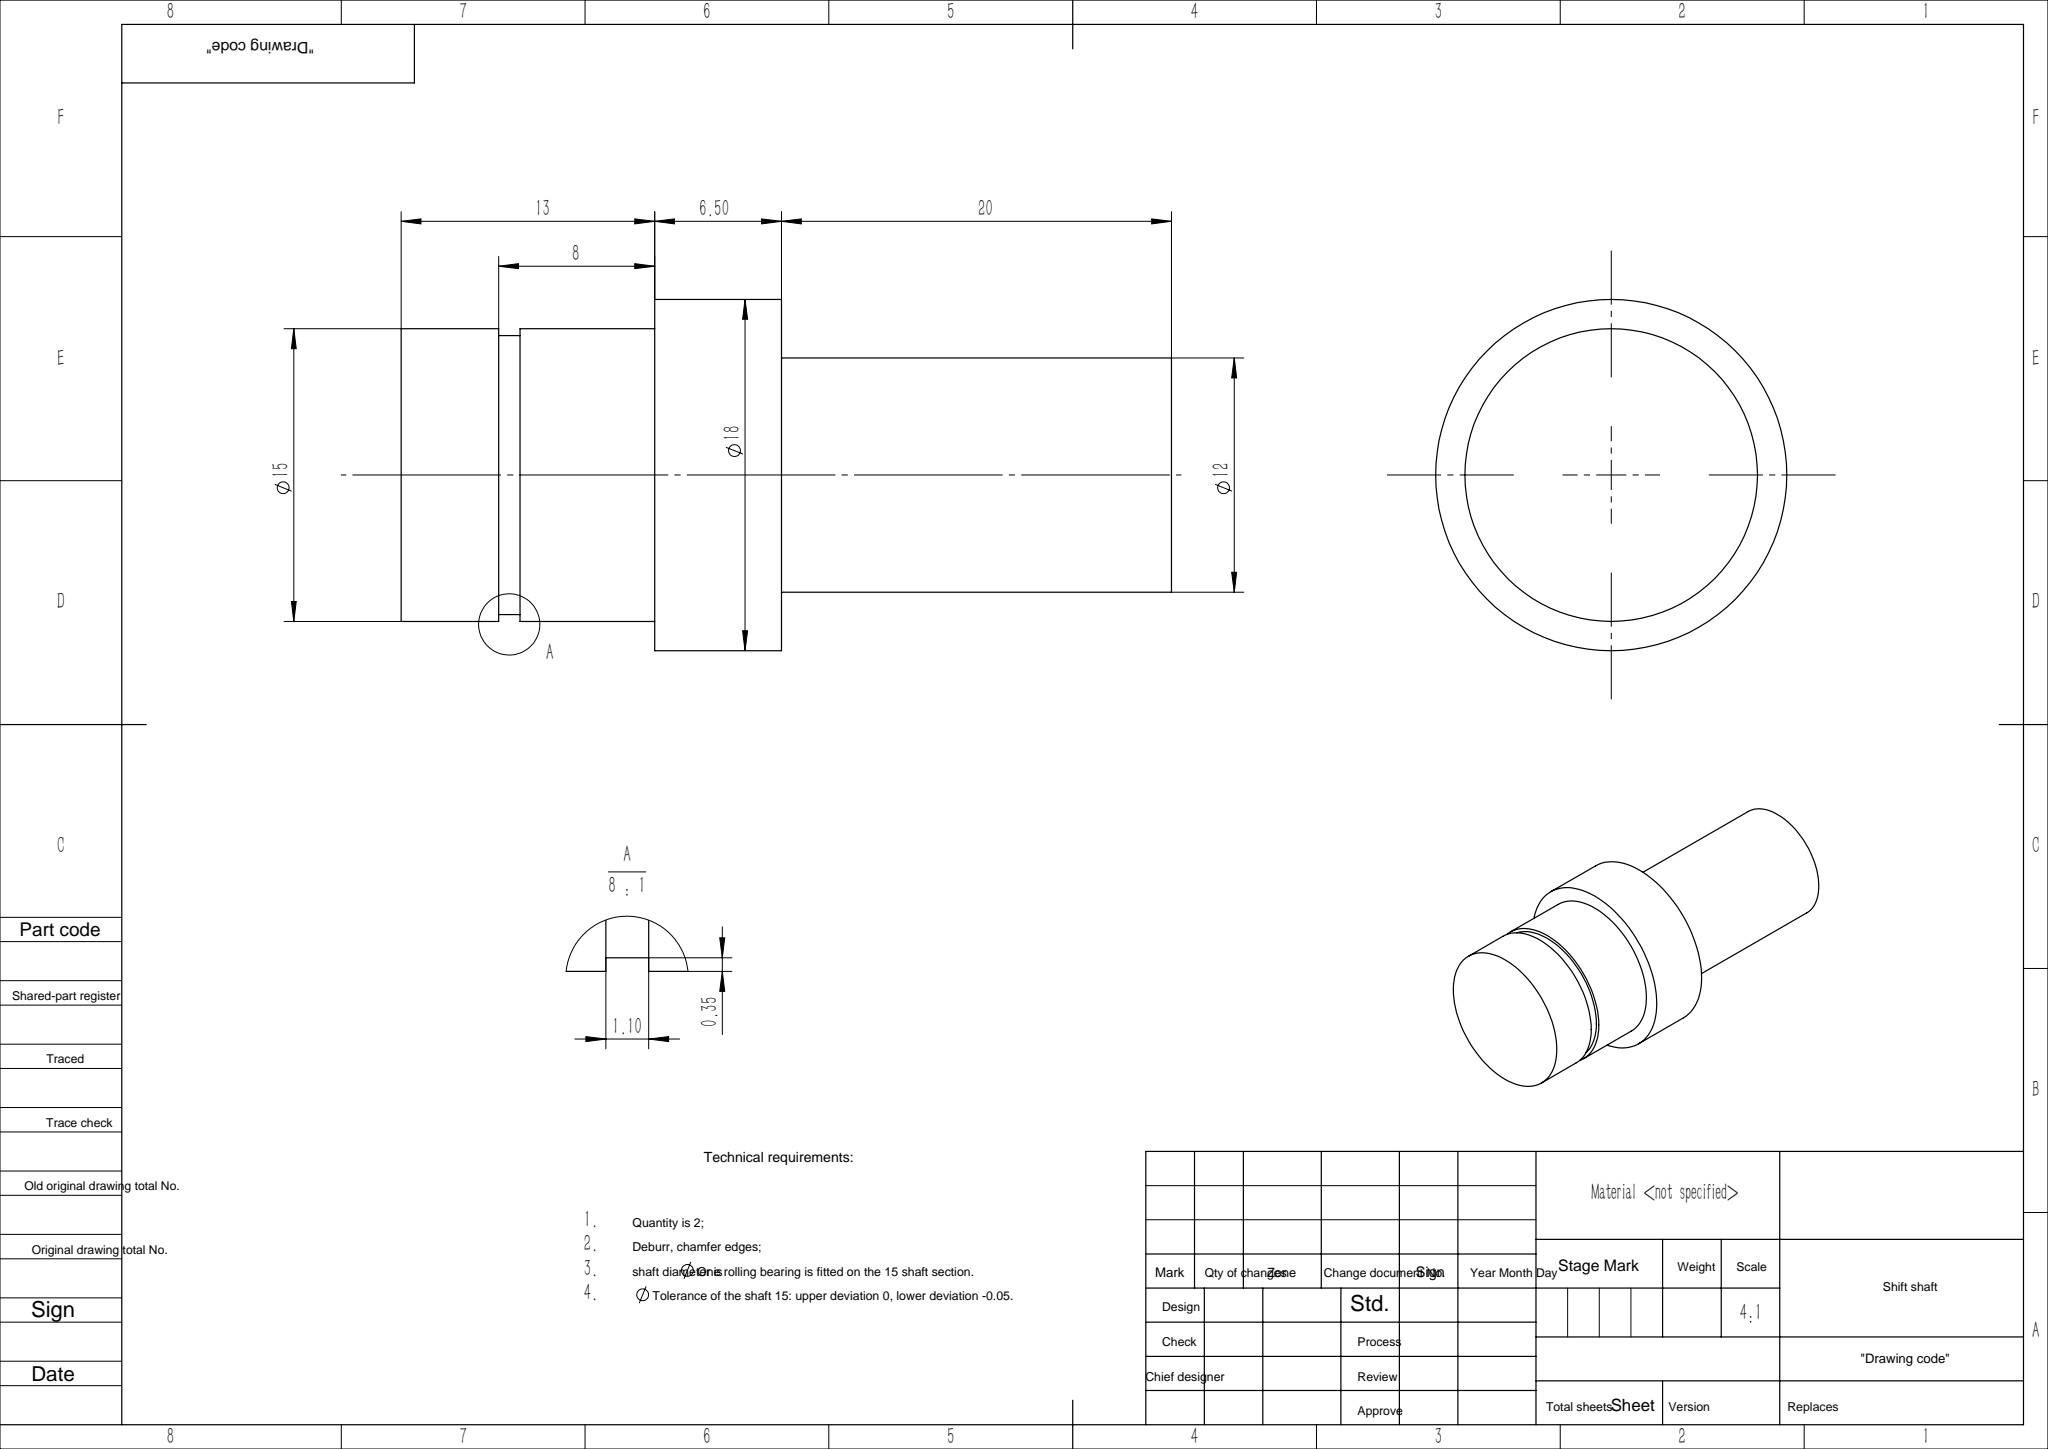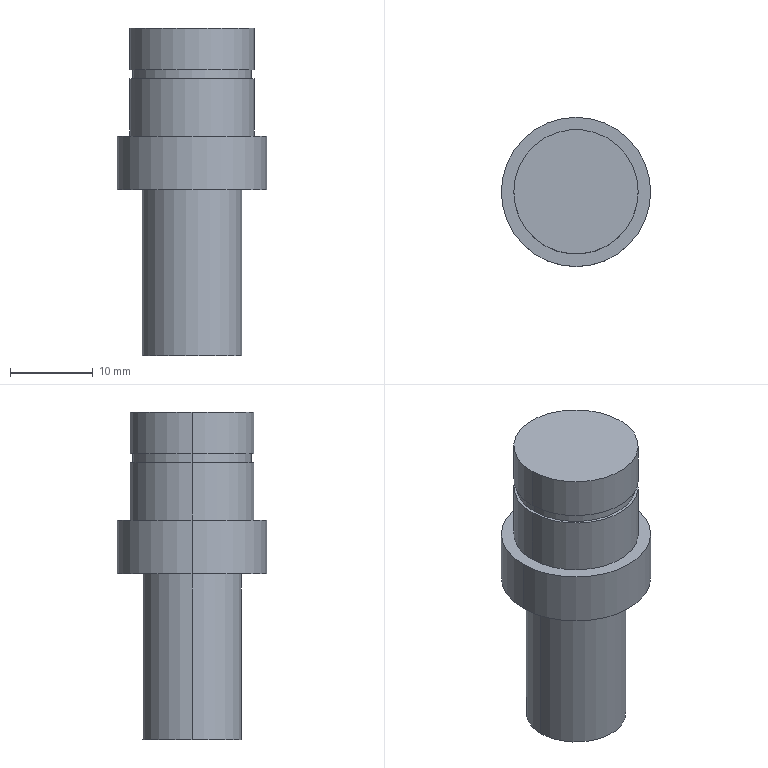Part | SolidWorks | features ICE 1, Revolution 1 | 1 solid | 16 faces | box 18 x 18 x 39.5 mm | volume 6196 mm3 | cylinder 10 | plane 6 | commonest cylinder face diameters 15 x4 12 x2 14.3 x2 18 x2
STEP:
#1=CARTESIAN_POINT('',(-7.5,0.,0.));
#2=VERTEX_POINT('',#1);
#3=CARTESIAN_POINT('',(7.5,0.,0.));
#4=VERTEX_POINT('',#3);
#5=CARTESIAN_POINT('',(0.,0.,0.));
#6=DIRECTION('',(0.,0.,-1.));
#7=DIRECTION('',(-1.,0.,0.));
#8=AXIS2_PLACEMENT_3D('',#5,#6,#7);
#9=CIRCLE('',#8,7.5);
#10=EDGE_CURVE('',#2,#4,#9,.T.);
#11=ORIENTED_EDGE('',*,*,#10,.T.);
#12=CARTESIAN_POINT('',(7.5,0.,-5.));
#13=VERTEX_POINT('',#12);
#14=CARTESIAN_POINT('',(7.5,0.,-39.5));
#15=DIRECTION('',(0.,0.,-1.));
#16=VECTOR('',#15,1000.);
#17=LINE('',#14,#16);
#18=EDGE_CURVE('',#4,#13,#17,.T.);
#19=ORIENTED_EDGE('',*,*,#18,.T.);
#20=CARTESIAN_POINT('',(-7.5,0.,-5.));
#21=VERTEX_POINT('',#20);
#22=CARTESIAN_POINT('',(0.,0.,-5.));
#23=DIRECTION('',(0.,0.,1.));
#24=DIRECTION('',(1.,0.,0.));
#25=AXIS2_PLACEMENT_3D('',#22,#23,#24);
#26=CIRCLE('',#25,7.5);
#27=EDGE_CURVE('',#13,#21,#26,.T.);
#28=ORIENTED_EDGE('',*,*,#27,.T.);
#29=CARTESIAN_POINT('',(-7.5,0.,-39.5));
#30=DIRECTION('',(0.,0.,-1.));
#31=VECTOR('',#30,1000.);
#32=LINE('',#29,#31);
#33=EDGE_CURVE('',#2,#21,#32,.T.);
#34=ORIENTED_EDGE('',*,*,#33,.F.);
#35=EDGE_LOOP('',(#11,#19,#28,#34));
#36=FACE_OUTER_BOUND('',#35,.T.);
#37=CARTESIAN_POINT('',(0.,0.,-39.5));
#38=DIRECTION('',(0.,0.,-1.));
#39=DIRECTION('',(-1.,0.,0.));
#40=AXIS2_PLACEMENT_3D('',#37,#38,#39);
#41=CYLINDRICAL_SURFACE('',#40,7.5);
#42=ADVANCED_FACE('',(#36),#41,.T.);
#43=CARTESIAN_POINT('',(7.15,0.,-6.1));
#44=VERTEX_POINT('',#43);
#45=CARTESIAN_POINT('',(-7.15,0.,-6.1));
#46=VERTEX_POINT('',#45);
#47=CARTESIAN_POINT('',(0.,0.,-6.1));
#48=DIRECTION('',(0.,0.,1.));
#49=DIRECTION('',(1.,0.,0.));
#50=AXIS2_PLACEMENT_3D('',#47,#48,#49);
#51=CIRCLE('',#50,7.15);
#52=EDGE_CURVE('',#44,#46,#51,.T.);
#53=ORIENTED_EDGE('',*,*,#52,.T.);
#54=CARTESIAN_POINT('',(-7.15,0.,-5.));
#55=VERTEX_POINT('',#54);
#56=CARTESIAN_POINT('',(-7.15,0.,-6.1));
#57=DIRECTION('',(0.,0.,1.));
#58=VECTOR('',#57,1000.);
#59=LINE('',#56,#58);
#60=EDGE_CURVE('',#46,#55,#59,.T.);
#61=ORIENTED_EDGE('',*,*,#60,.T.);
#62=CARTESIAN_POINT('',(7.15,0.,-5.));
#63=VERTEX_POINT('',#62);
#64=CARTESIAN_POINT('',(0.,0.,-5.));
#65=DIRECTION('',(0.,0.,1.));
#66=DIRECTION('',(1.,0.,0.));
#67=AXIS2_PLACEMENT_3D('',#64,#65,#66);
#68=CIRCLE('',#67,7.15);
#69=EDGE_CURVE('',#63,#55,#68,.T.);
#70=ORIENTED_EDGE('',*,*,#69,.F.);
#71=CARTESIAN_POINT('',(7.15,0.,-6.1));
#72=DIRECTION('',(0.,0.,1.));
#73=VECTOR('',#72,1000.);
#74=LINE('',#71,#73);
#75=EDGE_CURVE('',#44,#63,#74,.T.);
#76=ORIENTED_EDGE('',*,*,#75,.F.);
#77=EDGE_LOOP('',(#53,#61,#70,#76));
#78=FACE_OUTER_BOUND('',#77,.T.);
#79=CARTESIAN_POINT('',(0.,0.,-6.1));
#80=DIRECTION('',(0.,0.,1.));
#81=DIRECTION('',(1.,0.,0.));
#82=AXIS2_PLACEMENT_3D('',#79,#80,#81);
#83=CYLINDRICAL_SURFACE('',#82,7.15);
#84=ADVANCED_FACE('',(#78),#83,.T.);
#85=CARTESIAN_POINT('',(-6.,0.,-19.5));
#86=VERTEX_POINT('',#85);
#87=CARTESIAN_POINT('',(6.,0.,-19.5));
#88=VERTEX_POINT('',#87);
#89=CARTESIAN_POINT('',(0.,0.,-19.5));
#90=DIRECTION('',(0.,0.,-1.));
#91=DIRECTION('',(-1.,0.,0.));
#92=AXIS2_PLACEMENT_3D('',#89,#90,#91);
#93=CIRCLE('',#92,6.);
#94=EDGE_CURVE('',#86,#88,#93,.T.);
#95=ORIENTED_EDGE('',*,*,#94,.T.);
#96=CARTESIAN_POINT('',(6.,0.,-39.5));
#97=VERTEX_POINT('',#96);
#98=CARTESIAN_POINT('',(6.,0.,-39.5));
#99=DIRECTION('',(0.,0.,-1.));
#100=VECTOR('',#99,1000.);
#101=LINE('',#98,#100);
#102=EDGE_CURVE('',#88,#97,#101,.T.);
#103=ORIENTED_EDGE('',*,*,#102,.T.);
#104=CARTESIAN_POINT('',(-6.,0.,-39.5));
#105=VERTEX_POINT('',#104);
#106=CARTESIAN_POINT('',(0.,0.,-39.5));
#107=DIRECTION('',(0.,0.,-1.));
#108=DIRECTION('',(-1.,0.,0.));
#109=AXIS2_PLACEMENT_3D('',#106,#107,#108);
#110=CIRCLE('',#109,6.);
#111=EDGE_CURVE('',#105,#97,#110,.T.);
#112=ORIENTED_EDGE('',*,*,#111,.F.);
#113=CARTESIAN_POINT('',(-6.,0.,-39.5));
#114=DIRECTION('',(0.,0.,-1.));
#115=VECTOR('',#114,1000.);
#116=LINE('',#113,#115);
#117=EDGE_CURVE('',#86,#105,#116,.T.);
#118=ORIENTED_EDGE('',*,*,#117,.F.);
#119=EDGE_LOOP('',(#95,#103,#112,#118));
#120=FACE_OUTER_BOUND('',#119,.T.);
#121=CARTESIAN_POINT('',(0.,0.,-39.5));
#122=DIRECTION('',(0.,0.,-1.));
#123=DIRECTION('',(-1.,0.,0.));
#124=AXIS2_PLACEMENT_3D('',#121,#122,#123);
#125=CYLINDRICAL_SURFACE('',#124,6.);
#126=ADVANCED_FACE('',(#120),#125,.T.);
#127=CARTESIAN_POINT('',(-9.,0.,-13.));
#128=VERTEX_POINT('',#127);
#129=CARTESIAN_POINT('',(9.,0.,-13.));
#130=VERTEX_POINT('',#129);
#131=CARTESIAN_POINT('',(0.,0.,-13.));
#132=DIRECTION('',(0.,0.,-1.));
#133=DIRECTION('',(-1.,0.,0.));
#134=AXIS2_PLACEMENT_3D('',#131,#132,#133);
#135=CIRCLE('',#134,9.);
#136=EDGE_CURVE('',#128,#130,#135,.T.);
#137=ORIENTED_EDGE('',*,*,#136,.T.);
#138=CARTESIAN_POINT('',(9.,0.,-19.5));
#139=VERTEX_POINT('',#138);
#140=CARTESIAN_POINT('',(9.,0.,-39.5));
#141=DIRECTION('',(0.,0.,-1.));
#142=VECTOR('',#141,1000.);
#143=LINE('',#140,#142);
#144=EDGE_CURVE('',#130,#139,#143,.T.);
#145=ORIENTED_EDGE('',*,*,#144,.T.);
#146=CARTESIAN_POINT('',(-9.,0.,-19.5));
#147=VERTEX_POINT('',#146);
#148=CARTESIAN_POINT('',(0.,0.,-19.5));
#149=DIRECTION('',(0.,0.,-1.));
#150=DIRECTION('',(-1.,0.,0.));
#151=AXIS2_PLACEMENT_3D('',#148,#149,#150);
#152=CIRCLE('',#151,9.);
#153=EDGE_CURVE('',#147,#139,#152,.T.);
#154=ORIENTED_EDGE('',*,*,#153,.F.);
#155=CARTESIAN_POINT('',(-9.,0.,-39.5));
#156=DIRECTION('',(0.,0.,-1.));
#157=VECTOR('',#156,1000.);
#158=LINE('',#155,#157);
#159=EDGE_CURVE('',#128,#147,#158,.T.);
#160=ORIENTED_EDGE('',*,*,#159,.F.);
#161=EDGE_LOOP('',(#137,#145,#154,#160));
#162=FACE_OUTER_BOUND('',#161,.T.);
#163=CARTESIAN_POINT('',(0.,0.,-39.5));
#164=DIRECTION('',(0.,0.,-1.));
#165=DIRECTION('',(-1.,0.,0.));
#166=AXIS2_PLACEMENT_3D('',#163,#164,#165);
#167=CYLINDRICAL_SURFACE('',#166,9.);
#168=ADVANCED_FACE('',(#162),#167,.T.);
#169=CARTESIAN_POINT('',(7.5,0.,-6.1));
#170=VERTEX_POINT('',#169);
#171=CARTESIAN_POINT('',(-7.5,0.,-6.1));
#172=VERTEX_POINT('',#171);
#173=CARTESIAN_POINT('',(0.,0.,-6.1));
#174=DIRECTION('',(0.,0.,1.));
#175=DIRECTION('',(1.,0.,0.));
#176=AXIS2_PLACEMENT_3D('',#173,#174,#175);
#177=CIRCLE('',#176,7.5);
#178=EDGE_CURVE('',#170,#172,#177,.T.);
#179=ORIENTED_EDGE('',*,*,#178,.F.);
#180=CARTESIAN_POINT('',(7.5,0.,-13.));
#181=VERTEX_POINT('',#180);
#182=CARTESIAN_POINT('',(7.5,0.,-39.5));
#183=DIRECTION('',(0.,0.,-1.));
#184=VECTOR('',#183,1000.);
#185=LINE('',#182,#184);
#186=EDGE_CURVE('',#170,#181,#185,.T.);
#187=ORIENTED_EDGE('',*,*,#186,.T.);
#188=CARTESIAN_POINT('',(-7.5,0.,-13.));
#189=VERTEX_POINT('',#188);
#190=CARTESIAN_POINT('',(0.,0.,-13.));
#191=DIRECTION('',(0.,0.,-1.));
#192=DIRECTION('',(-1.,0.,0.));
#193=AXIS2_PLACEMENT_3D('',#190,#191,#192);
#194=CIRCLE('',#193,7.5);
#195=EDGE_CURVE('',#189,#181,#194,.T.);
#196=ORIENTED_EDGE('',*,*,#195,.F.);
#197=CARTESIAN_POINT('',(-7.5,0.,-39.5));
#198=DIRECTION('',(0.,0.,-1.));
#199=VECTOR('',#198,1000.);
#200=LINE('',#197,#199);
#201=EDGE_CURVE('',#172,#189,#200,.T.);
#202=ORIENTED_EDGE('',*,*,#201,.F.);
#203=EDGE_LOOP('',(#179,#187,#196,#202));
#204=FACE_OUTER_BOUND('',#203,.T.);
#205=CARTESIAN_POINT('',(0.,0.,-39.5));
#206=DIRECTION('',(0.,0.,-1.));
#207=DIRECTION('',(-1.,0.,0.));
#208=AXIS2_PLACEMENT_3D('',#205,#206,#207);
#209=CYLINDRICAL_SURFACE('',#208,7.5);
#210=ADVANCED_FACE('',(#204),#209,.T.);
#211=ORIENTED_EDGE('',*,*,#186,.F.);
#212=CARTESIAN_POINT('',(0.,0.,-6.1));
#213=DIRECTION('',(0.,0.,1.));
#214=DIRECTION('',(1.,0.,0.));
#215=AXIS2_PLACEMENT_3D('',#212,#213,#214);
#216=CIRCLE('',#215,7.5);
#217=EDGE_CURVE('',#172,#170,#216,.T.);
#218=ORIENTED_EDGE('',*,*,#217,.F.);
#219=ORIENTED_EDGE('',*,*,#201,.T.);
#220=CARTESIAN_POINT('',(0.,0.,-13.));
#221=DIRECTION('',(0.,0.,-1.));
#222=DIRECTION('',(-1.,0.,0.));
#223=AXIS2_PLACEMENT_3D('',#220,#221,#222);
#224=CIRCLE('',#223,7.5);
#225=EDGE_CURVE('',#181,#189,#224,.T.);
#226=ORIENTED_EDGE('',*,*,#225,.F.);
#227=EDGE_LOOP('',(#211,#218,#219,#226));
#228=FACE_OUTER_BOUND('',#227,.T.);
#229=CARTESIAN_POINT('',(0.,0.,-39.5));
#230=DIRECTION('',(0.,0.,-1.));
#231=DIRECTION('',(-1.,0.,0.));
#232=AXIS2_PLACEMENT_3D('',#229,#230,#231);
#233=CYLINDRICAL_SURFACE('',#232,7.5);
#234=ADVANCED_FACE('',(#228),#233,.T.);
#235=ORIENTED_EDGE('',*,*,#195,.T.);
#236=ORIENTED_EDGE('',*,*,#225,.T.);
#237=EDGE_LOOP('',(#235,#236));
#238=FACE_BOUND('',#237,.T.);
#239=ORIENTED_EDGE('',*,*,#136,.F.);
#240=CARTESIAN_POINT('',(0.,0.,-13.));
#241=DIRECTION('',(0.,0.,-1.));
#242=DIRECTION('',(-1.,0.,0.));
#243=AXIS2_PLACEMENT_3D('',#240,#241,#242);
#244=CIRCLE('',#243,9.);
#245=EDGE_CURVE('',#130,#128,#244,.T.);
#246=ORIENTED_EDGE('',*,*,#245,.F.);
#247=EDGE_LOOP('',(#239,#246));
#248=FACE_OUTER_BOUND('',#247,.T.);
#249=CARTESIAN_POINT('',(0.,7.5,-13.));
#250=DIRECTION('',(0.,0.,1.));
#251=DIRECTION('',(1.,0.,0.));
#252=AXIS2_PLACEMENT_3D('',#249,#250,#251);
#253=PLANE('',#252);
#254=ADVANCED_FACE('',(#238,#248),#253,.T.);
#255=ORIENTED_EDGE('',*,*,#144,.F.);
#256=ORIENTED_EDGE('',*,*,#245,.T.);
#257=ORIENTED_EDGE('',*,*,#159,.T.);
#258=CARTESIAN_POINT('',(0.,0.,-19.5));
#259=DIRECTION('',(0.,0.,-1.));
#260=DIRECTION('',(-1.,0.,0.));
#261=AXIS2_PLACEMENT_3D('',#258,#259,#260);
#262=CIRCLE('',#261,9.);
#263=EDGE_CURVE('',#139,#147,#262,.T.);
#264=ORIENTED_EDGE('',*,*,#263,.F.);
#265=EDGE_LOOP('',(#255,#256,#257,#264));
#266=FACE_OUTER_BOUND('',#265,.T.);
#267=CARTESIAN_POINT('',(0.,0.,-39.5));
#268=DIRECTION('',(0.,0.,-1.));
#269=DIRECTION('',(-1.,0.,0.));
#270=AXIS2_PLACEMENT_3D('',#267,#268,#269);
#271=CYLINDRICAL_SURFACE('',#270,9.);
#272=ADVANCED_FACE('',(#266),#271,.T.);
#273=ORIENTED_EDGE('',*,*,#153,.T.);
#274=ORIENTED_EDGE('',*,*,#263,.T.);
#275=EDGE_LOOP('',(#273,#274));
#276=FACE_OUTER_BOUND('',#275,.T.);
#277=ORIENTED_EDGE('',*,*,#94,.F.);
#278=CARTESIAN_POINT('',(0.,0.,-19.5));
#279=DIRECTION('',(0.,0.,-1.));
#280=DIRECTION('',(-1.,0.,0.));
#281=AXIS2_PLACEMENT_3D('',#278,#279,#280);
#282=CIRCLE('',#281,6.);
#283=EDGE_CURVE('',#88,#86,#282,.T.);
#284=ORIENTED_EDGE('',*,*,#283,.F.);
#285=EDGE_LOOP('',(#277,#284));
#286=FACE_BOUND('',#285,.T.);
#287=CARTESIAN_POINT('',(0.,9.,-19.5));
#288=DIRECTION('',(0.,0.,-1.));
#289=DIRECTION('',(-1.,0.,0.));
#290=AXIS2_PLACEMENT_3D('',#287,#288,#289);
#291=PLANE('',#290);
#292=ADVANCED_FACE('',(#276,#286),#291,.T.);
#293=ORIENTED_EDGE('',*,*,#102,.F.);
#294=ORIENTED_EDGE('',*,*,#283,.T.);
#295=ORIENTED_EDGE('',*,*,#117,.T.);
#296=CARTESIAN_POINT('',(0.,0.,-39.5));
#297=DIRECTION('',(0.,0.,-1.));
#298=DIRECTION('',(-1.,0.,0.));
#299=AXIS2_PLACEMENT_3D('',#296,#297,#298);
#300=CIRCLE('',#299,6.);
#301=EDGE_CURVE('',#97,#105,#300,.T.);
#302=ORIENTED_EDGE('',*,*,#301,.F.);
#303=EDGE_LOOP('',(#293,#294,#295,#302));
#304=FACE_OUTER_BOUND('',#303,.T.);
#305=CARTESIAN_POINT('',(0.,0.,-39.5));
#306=DIRECTION('',(0.,0.,-1.));
#307=DIRECTION('',(-1.,0.,0.));
#308=AXIS2_PLACEMENT_3D('',#305,#306,#307);
#309=CYLINDRICAL_SURFACE('',#308,6.);
#310=ADVANCED_FACE('',(#304),#309,.T.);
#311=ORIENTED_EDGE('',*,*,#111,.T.);
#312=ORIENTED_EDGE('',*,*,#301,.T.);
#313=EDGE_LOOP('',(#311,#312));
#314=FACE_OUTER_BOUND('',#313,.T.);
#315=CARTESIAN_POINT('',(0.,6.,-39.5));
#316=DIRECTION('',(0.,0.,-1.));
#317=DIRECTION('',(-1.,0.,0.));
#318=AXIS2_PLACEMENT_3D('',#315,#316,#317);
#319=PLANE('',#318);
#320=ADVANCED_FACE('',(#314),#319,.T.);
#321=ORIENTED_EDGE('',*,*,#52,.F.);
#322=CARTESIAN_POINT('',(0.,0.,-6.1));
#323=DIRECTION('',(0.,0.,1.));
#324=DIRECTION('',(1.,0.,0.));
#325=AXIS2_PLACEMENT_3D('',#322,#323,#324);
#326=CIRCLE('',#325,7.15);
#327=EDGE_CURVE('',#46,#44,#326,.T.);
#328=ORIENTED_EDGE('',*,*,#327,.F.);
#329=EDGE_LOOP('',(#321,#328));
#330=FACE_BOUND('',#329,.T.);
#331=ORIENTED_EDGE('',*,*,#217,.T.);
#332=ORIENTED_EDGE('',*,*,#178,.T.);
#333=EDGE_LOOP('',(#331,#332));
#334=FACE_OUTER_BOUND('',#333,.T.);
#335=CARTESIAN_POINT('',(0.,0.,-6.1));
#336=DIRECTION('',(0.,0.,1.));
#337=DIRECTION('',(1.,0.,0.));
#338=AXIS2_PLACEMENT_3D('',#335,#336,#337);
#339=PLANE('',#338);
#340=ADVANCED_FACE('',(#330,#334),#339,.T.);
#341=ORIENTED_EDGE('',*,*,#69,.T.);
#342=CARTESIAN_POINT('',(0.,0.,-5.));
#343=DIRECTION('',(0.,0.,1.));
#344=DIRECTION('',(1.,0.,0.));
#345=AXIS2_PLACEMENT_3D('',#342,#343,#344);
#346=CIRCLE('',#345,7.15);
#347=EDGE_CURVE('',#55,#63,#346,.T.);
#348=ORIENTED_EDGE('',*,*,#347,.T.);
#349=EDGE_LOOP('',(#341,#348));
#350=FACE_BOUND('',#349,.T.);
#351=CARTESIAN_POINT('',(0.,0.,-5.));
#352=DIRECTION('',(0.,0.,1.));
#353=DIRECTION('',(1.,0.,0.));
#354=AXIS2_PLACEMENT_3D('',#351,#352,#353);
#355=CIRCLE('',#354,7.5);
#356=EDGE_CURVE('',#21,#13,#355,.T.);
#357=ORIENTED_EDGE('',*,*,#356,.F.);
#358=ORIENTED_EDGE('',*,*,#27,.F.);
#359=EDGE_LOOP('',(#357,#358));
#360=FACE_OUTER_BOUND('',#359,.T.);
#361=CARTESIAN_POINT('',(0.,0.,-5.));
#362=DIRECTION('',(0.,0.,1.));
#363=DIRECTION('',(1.,0.,0.));
#364=AXIS2_PLACEMENT_3D('',#361,#362,#363);
#365=PLANE('',#364);
#366=ADVANCED_FACE('',(#350,#360),#365,.F.);
#367=ORIENTED_EDGE('',*,*,#60,.F.);
#368=ORIENTED_EDGE('',*,*,#327,.T.);
#369=ORIENTED_EDGE('',*,*,#75,.T.);
#370=ORIENTED_EDGE('',*,*,#347,.F.);
#371=EDGE_LOOP('',(#367,#368,#369,#370));
#372=FACE_OUTER_BOUND('',#371,.T.);
#373=CARTESIAN_POINT('',(0.,0.,-6.1));
#374=DIRECTION('',(0.,0.,1.));
#375=DIRECTION('',(1.,0.,0.));
#376=AXIS2_PLACEMENT_3D('',#373,#374,#375);
#377=CYLINDRICAL_SURFACE('',#376,7.15);
#378=ADVANCED_FACE('',(#372),#377,.T.);
#379=ORIENTED_EDGE('',*,*,#10,.F.);
#380=CARTESIAN_POINT('',(0.,0.,0.));
#381=DIRECTION('',(0.,0.,-1.));
#382=DIRECTION('',(-1.,0.,0.));
#383=AXIS2_PLACEMENT_3D('',#380,#381,#382);
#384=CIRCLE('',#383,7.5);
#385=EDGE_CURVE('',#4,#2,#384,.T.);
#386=ORIENTED_EDGE('',*,*,#385,.F.);
#387=EDGE_LOOP('',(#379,#386));
#388=FACE_OUTER_BOUND('',#387,.T.);
#389=CARTESIAN_POINT('',(0.,0.,0.));
#390=DIRECTION('',(0.,0.,1.));
#391=DIRECTION('',(1.,0.,0.));
#392=AXIS2_PLACEMENT_3D('',#389,#390,#391);
#393=PLANE('',#392);
#394=ADVANCED_FACE('',(#388),#393,.T.);
#395=ORIENTED_EDGE('',*,*,#18,.F.);
#396=ORIENTED_EDGE('',*,*,#385,.T.);
#397=ORIENTED_EDGE('',*,*,#33,.T.);
#398=ORIENTED_EDGE('',*,*,#356,.T.);
#399=EDGE_LOOP('',(#395,#396,#397,#398));
#400=FACE_OUTER_BOUND('',#399,.T.);
#401=CARTESIAN_POINT('',(0.,0.,-39.5));
#402=DIRECTION('',(0.,0.,-1.));
#403=DIRECTION('',(-1.,0.,0.));
#404=AXIS2_PLACEMENT_3D('',#401,#402,#403);
#405=CYLINDRICAL_SURFACE('',#404,7.5);
#406=ADVANCED_FACE('',(#400),#405,.T.);
#407=CLOSED_SHELL('',(#42,#84,#126,#168,#210,#234,#254,#272,#292,#310,#320,#340,#366,#378,#394,#406));
#408=MANIFOLD_SOLID_BREP('',#407);
#409=CARTESIAN_POINT('',(0.,0.,0.));
#410=DIRECTION('',(0.,0.,1.));
#411=DIRECTION('',(1.,0.,0.));
#412=AXIS2_PLACEMENT_3D('',#409,#410,#411);
#413=(LENGTH_UNIT()NAMED_UNIT(*)SI_UNIT(.MILLI.,.METRE.));
#414=UNCERTAINTY_MEASURE_WITH_UNIT(LENGTH_MEASURE(0.00001),#413,'','');
#415=(NAMED_UNIT(*)PLANE_ANGLE_UNIT()SI_UNIT($,.RADIAN.));
#416=(NAMED_UNIT(*)SI_UNIT($,.STERADIAN.)SOLID_ANGLE_UNIT());
#417=(GEOMETRIC_REPRESENTATION_CONTEXT(3)GLOBAL_UNCERTAINTY_ASSIGNED_CONTEXT((#414))GLOBAL_UNIT_ASSIGNED_CONTEXT((#413,#415,#416))REPRESENTATION_CONTEXT('',''));
#418=ADVANCED_BREP_SHAPE_REPRESENTATION('',(#408,#412),#417);